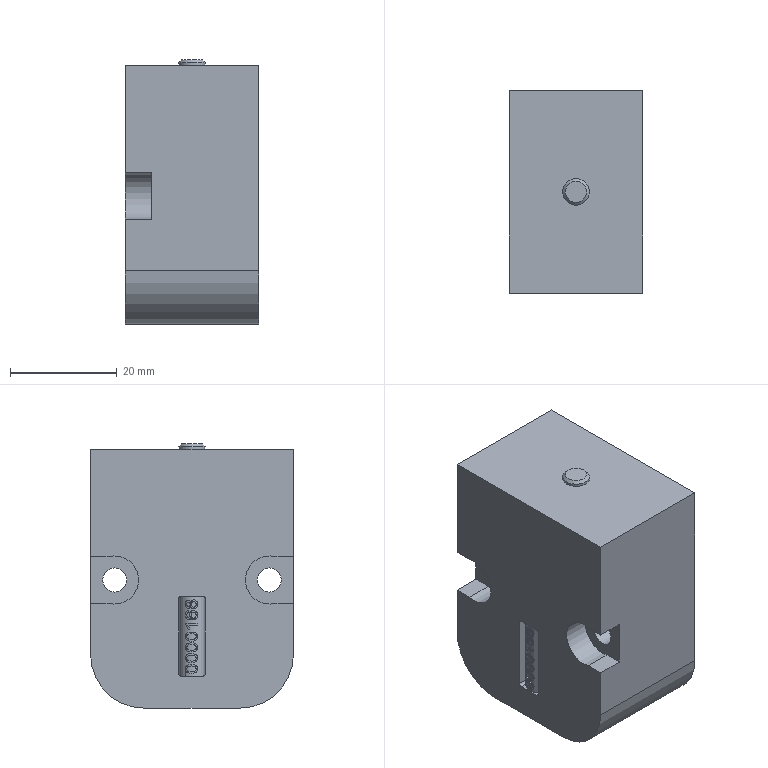Part | STEP file | solid 13 | 1 solid | 135 faces | box 25 x 38 x 49.5 mm | volume 43620 mm3 | other 83 | plane 25 | cylinder 19 | spline 7 | cone 1 | commonest cylinder face diameters 4.8 x8 1 x4 4.5 x2 9 x2 20 x2 5 x1